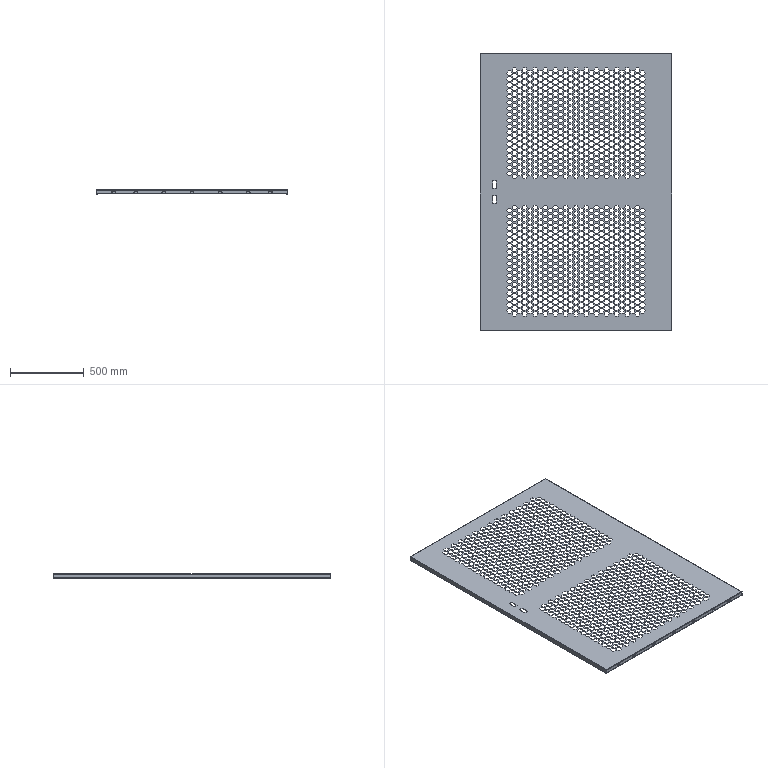Part | SolidWorks | features BaseBody 1 | 1 solid | 6190 faces | volume 3836905 mm3 | plane 6138 | cylinder 52 | commonest cylinder face diameters 10 x14 12 x14 2 x10 6 x10 0.1 x2 4.1 x2